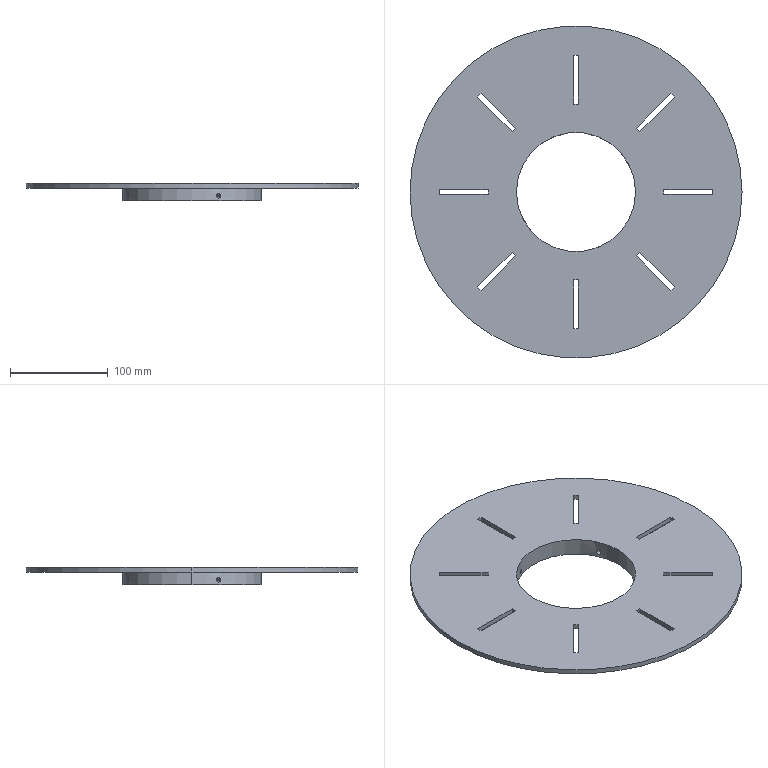Part | SolidWorks | features CirPattern 2, ICE 2, Extrusion 1, RevCut 1 | 1 solid | 49 faces | box 340 x 340 x 18 mm | volume 438812 mm3 | plane 35 | cylinder 14 | commonest cylinder face diameters 4.4 x8 122 x2 142 x2 340 x2